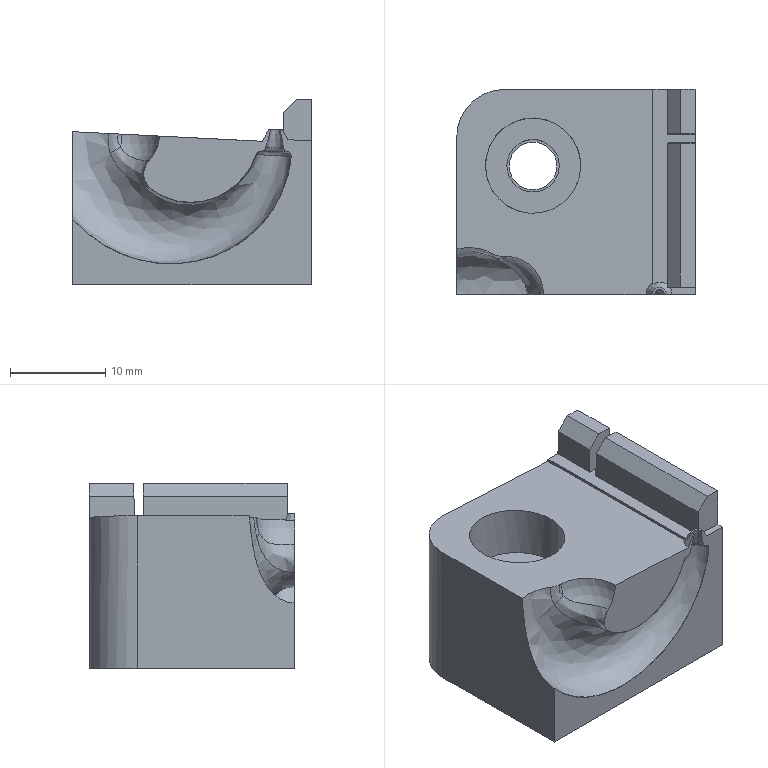Part | STEP file | solid 195 | 1 solid | 41 faces | box 25 x 21.5 x 19.435 mm | volume 7243 mm3 | plane 17 | spline 15 | cylinder 7 | cone 1 | sphere 1 | commonest cylinder face diameters 10 x2 6922 x2 5 x1 5.5 x1 8 x1